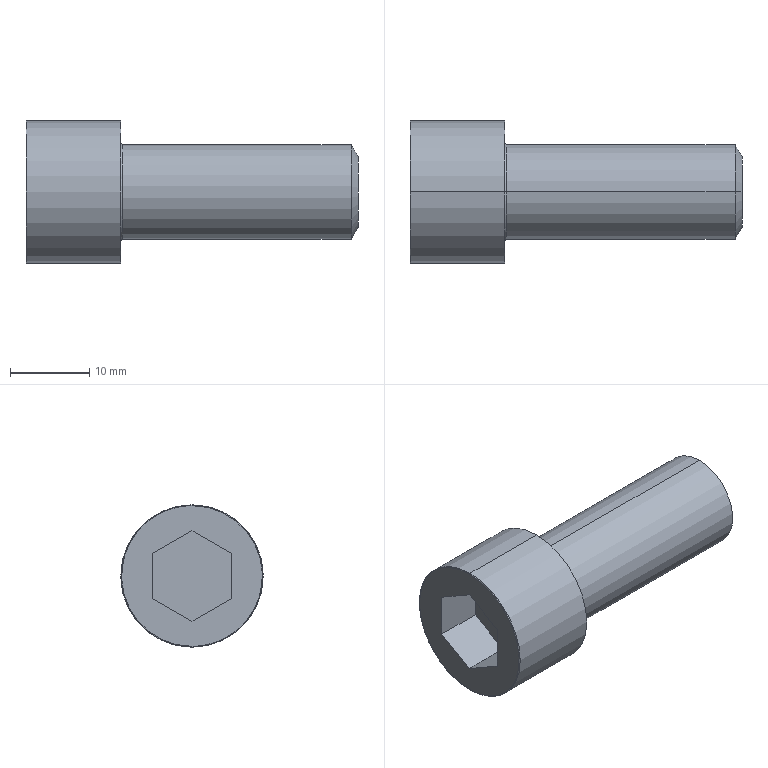Part | STEP file | 1 solid | 20 faces | box 42 x 18 x 18 mm | volume 5915 mm3 | plane 10 | spline 4 | cylinder 4 | cone 2 | commonest cylinder face diameters 12 x2 18 x2